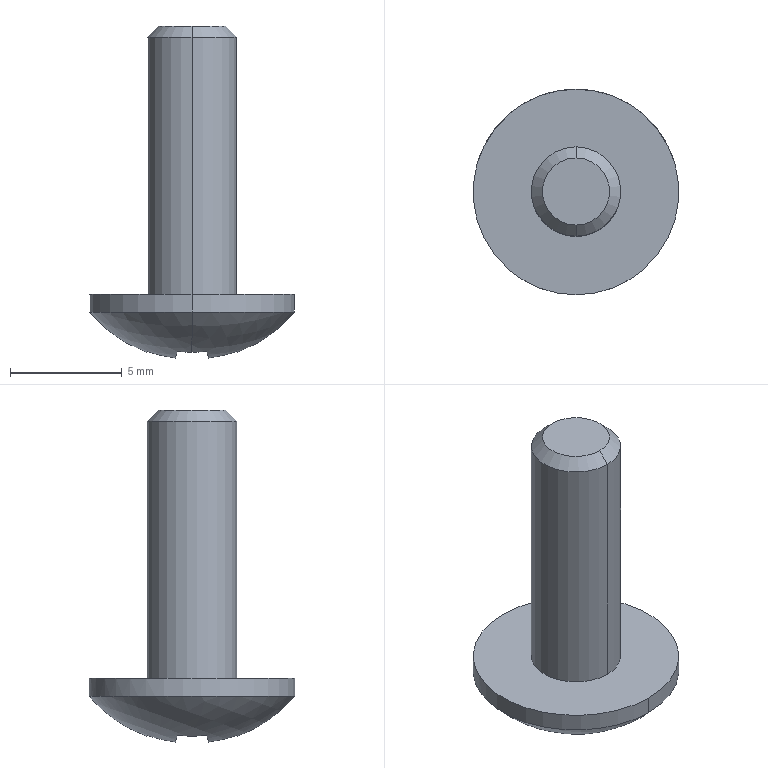Part | STEP file | MSBR-15_1_1_1_1 | 1 solid | 23 faces | box 9.2 x 9.2 x 14.856 mm | volume 268.703 mm3 | plane 15 | cylinder 4 | sphere 2 | cone 2 | commonest cylinder face diameters 4 x2 9.2 x2
STEP:
#1=CARTESIAN_POINT('',(0.,0.,0.));
#2=DIRECTION('',(0.,0.,1.));
#3=DIRECTION('',(1.,0.,0.));
#4=AXIS2_PLACEMENT_3D('',#1,#2,#3);
#5=CARTESIAN_POINT('',(0.,4.6,-18.7));
#6=VERTEX_POINT('',#5);
#7=CARTESIAN_POINT('',(0.,-4.6,-18.7));
#8=VERTEX_POINT('',#7);
#9=CARTESIAN_POINT('',(0.,0.,-18.7));
#10=DIRECTION('',(0.,0.,-1.));
#11=DIRECTION('',(0.,1.,0.));
#12=AXIS2_PLACEMENT_3D('',#9,#10,#11);
#13=CIRCLE('',#12,4.6);
#14=EDGE_CURVE('',#6,#8,#13,.T.);
#15=ORIENTED_EDGE('',*,*,#14,.F.);
#16=CARTESIAN_POINT('',(0.,4.6,-19.5));
#17=VERTEX_POINT('',#16);
#18=CARTESIAN_POINT('',(0.,4.6,-19.5));
#19=DIRECTION('',(0.,-0.000000001,1.));
#20=VECTOR('',#19,0.8);
#21=LINE('',#18,#20);
#22=EDGE_CURVE('',#17,#6,#21,.T.);
#23=ORIENTED_EDGE('',*,*,#22,.F.);
#24=CARTESIAN_POINT('',(0.,-4.6,-19.5));
#25=VERTEX_POINT('',#24);
#26=CARTESIAN_POINT('',(0.,0.,-19.5));
#27=DIRECTION('',(0.,0.,1.));
#28=DIRECTION('',(0.,-1.,0.));
#29=AXIS2_PLACEMENT_3D('',#26,#27,#28);
#30=CIRCLE('',#29,4.6);
#31=EDGE_CURVE('',#25,#17,#30,.T.);
#32=ORIENTED_EDGE('',*,*,#31,.F.);
#33=CARTESIAN_POINT('',(0.,-4.6,-18.7));
#34=DIRECTION('',(0.,-0.000000001,-1.));
#35=VECTOR('',#34,0.8);
#36=LINE('',#33,#35);
#37=EDGE_CURVE('',#8,#25,#36,.T.);
#38=ORIENTED_EDGE('',*,*,#37,.F.);
#39=EDGE_LOOP('',(#15,#23,#32,#38));
#40=FACE_OUTER_BOUND('',#39,.F.);
#41=CARTESIAN_POINT('',(0.,0.,-18.676));
#42=DIRECTION('',(0.,0.,-1.));
#43=DIRECTION('',(0.,1.,0.));
#44=AXIS2_PLACEMENT_3D('',#41,#42,#43);
#45=CYLINDRICAL_SURFACE('',#44,4.6);
#46=ADVANCED_FACE('',(#40),#45,.T.);
#47=CARTESIAN_POINT('',(0.,0.,-18.7));
#48=DIRECTION('',(0.,0.,-1.));
#49=DIRECTION('',(0.,-1.,0.));
#50=AXIS2_PLACEMENT_3D('',#47,#48,#49);
#51=CIRCLE('',#50,4.6);
#52=EDGE_CURVE('',#8,#6,#51,.T.);
#53=ORIENTED_EDGE('',*,*,#52,.T.);
#54=ORIENTED_EDGE('',*,*,#14,.T.);
#55=EDGE_LOOP('',(#53,#54));
#56=FACE_OUTER_BOUND('',#55,.F.);
#57=CARTESIAN_POINT('',(0.,-2.,-18.7));
#58=VERTEX_POINT('',#57);
#59=CARTESIAN_POINT('',(0.,2.,-18.7));
#60=VERTEX_POINT('',#59);
#61=CARTESIAN_POINT('',(0.,0.,-18.7));
#62=DIRECTION('',(0.,0.,1.));
#63=DIRECTION('',(0.,-1.,0.));
#64=AXIS2_PLACEMENT_3D('',#61,#62,#63);
#65=CIRCLE('',#64,2.);
#66=EDGE_CURVE('',#58,#60,#65,.T.);
#67=ORIENTED_EDGE('',*,*,#66,.T.);
#68=CARTESIAN_POINT('',(0.,0.,-18.7));
#69=DIRECTION('',(0.,0.,1.));
#70=DIRECTION('',(0.,1.,0.));
#71=AXIS2_PLACEMENT_3D('',#68,#69,#70);
#72=CIRCLE('',#71,2.);
#73=EDGE_CURVE('',#60,#58,#72,.T.);
#74=ORIENTED_EDGE('',*,*,#73,.T.);
#75=EDGE_LOOP('',(#67,#74));
#76=FACE_BOUND('',#75,.F.);
#77=CARTESIAN_POINT('',(0.,0.,-18.7));
#78=DIRECTION('',(0.,0.,1.));
#79=DIRECTION('',(0.,-1.,0.));
#80=AXIS2_PLACEMENT_3D('',#77,#78,#79);
#81=PLANE('',#80);
#82=ADVANCED_FACE('',(#56,#76),#81,.T.);
#83=ORIENTED_EDGE('',*,*,#37,.T.);
#84=CARTESIAN_POINT('',(0.,0.,-19.5));
#85=DIRECTION('',(0.,0.,1.));
#86=DIRECTION('',(0.,1.,0.));
#87=AXIS2_PLACEMENT_3D('',#84,#85,#86);
#88=CIRCLE('',#87,4.6);
#89=EDGE_CURVE('',#17,#25,#88,.T.);
#90=ORIENTED_EDGE('',*,*,#89,.F.);
#91=ORIENTED_EDGE('',*,*,#22,.T.);
#92=ORIENTED_EDGE('',*,*,#52,.F.);
#93=EDGE_LOOP('',(#83,#90,#91,#92));
#94=FACE_OUTER_BOUND('',#93,.F.);
#95=CARTESIAN_POINT('',(0.,0.,-18.676));
#96=DIRECTION('',(0.,0.,-1.));
#97=DIRECTION('',(0.,-1.,0.));
#98=AXIS2_PLACEMENT_3D('',#95,#96,#97);
#99=CYLINDRICAL_SURFACE('',#98,4.6);
#100=ADVANCED_FACE('',(#94),#99,.T.);
#101=ORIENTED_EDGE('',*,*,#89,.T.);
#102=CARTESIAN_POINT('',(0.,-2.03,-21.294));
#103=VERTEX_POINT('',#102);
#104=CARTESIAN_POINT('',(0.,0.,-15.648));
#105=DIRECTION('',(-1.,0.,0.));
#106=DIRECTION('',(0.,-0.3383,-0.941));
#107=AXIS2_PLACEMENT_3D('',#104,#105,#106);
#108=CIRCLE('',#107,6.);
#109=EDGE_CURVE('',#103,#25,#108,.T.);
#110=ORIENTED_EDGE('',*,*,#109,.F.);
#111=CARTESIAN_POINT('',(-0.669,-2.007,-21.262));
#112=VERTEX_POINT('',#111);
#113=CARTESIAN_POINT('',(0.,1.341,-16.613));
#114=DIRECTION('',(0.,-0.8115,0.5843));
#115=DIRECTION('',(-0.116,-0.5804,-0.8061));
#116=AXIS2_PLACEMENT_3D('',#113,#114,#115);
#117=CIRCLE('',#116,5.768);
#118=EDGE_CURVE('',#112,#103,#117,.T.);
#119=ORIENTED_EDGE('',*,*,#118,.F.);
#120=CARTESIAN_POINT('',(-0.7394,-0.7394,-21.556));
#121=VERTEX_POINT('',#120);
#122=CARTESIAN_POINT('',(0.6416,0.,-15.802));
#123=DIRECTION('',(-0.9724,0.,0.2334));
#124=DIRECTION('',(-0.2316,-0.124,-0.9649));
#125=AXIS2_PLACEMENT_3D('',#122,#123,#124);
#126=CIRCLE('',#125,5.964);
#127=EDGE_CURVE('',#121,#112,#126,.T.);
#128=ORIENTED_EDGE('',*,*,#127,.F.);
#129=CARTESIAN_POINT('',(-2.007,-0.669,-21.262));
#130=VERTEX_POINT('',#129);
#131=CARTESIAN_POINT('',(0.,0.6416,-15.802));
#132=DIRECTION('',(0.,-0.9724,0.2334));
#133=DIRECTION('',(-0.3365,-0.2198,-0.9157));
#134=AXIS2_PLACEMENT_3D('',#131,#132,#133);
#135=CIRCLE('',#134,5.964);
#136=EDGE_CURVE('',#130,#121,#135,.T.);
#137=ORIENTED_EDGE('',*,*,#136,.F.);
#138=CARTESIAN_POINT('',(-2.007,0.669,-21.262));
#139=VERTEX_POINT('',#138);
#140=CARTESIAN_POINT('',(1.341,0.,-16.613));
#141=DIRECTION('',(-0.8115,0.,0.5843));
#142=DIRECTION('',(-0.5804,0.116,-0.8061));
#143=AXIS2_PLACEMENT_3D('',#140,#141,#142);
#144=CIRCLE('',#143,5.768);
#145=EDGE_CURVE('',#139,#130,#144,.T.);
#146=ORIENTED_EDGE('',*,*,#145,.F.);
#147=CARTESIAN_POINT('',(-0.7394,0.7394,-21.556));
#148=VERTEX_POINT('',#147);
#149=CARTESIAN_POINT('',(0.,-0.6416,-15.802));
#150=DIRECTION('',(0.,-0.9724,-0.2334));
#151=DIRECTION('',(-0.3365,0.2198,-0.9157));
#152=AXIS2_PLACEMENT_3D('',#149,#150,#151);
#153=CIRCLE('',#152,5.964);
#154=EDGE_CURVE('',#139,#148,#153,.T.);
#155=ORIENTED_EDGE('',*,*,#154,.T.);
#156=CARTESIAN_POINT('',(-0.669,2.007,-21.262));
#157=VERTEX_POINT('',#156);
#158=CARTESIAN_POINT('',(0.6416,0.,-15.802));
#159=DIRECTION('',(0.9724,0.,-0.2334));
#160=DIRECTION('',(-0.2316,0.124,-0.9649));
#161=AXIS2_PLACEMENT_3D('',#158,#159,#160);
#162=CIRCLE('',#161,5.964);
#163=EDGE_CURVE('',#148,#157,#162,.T.);
#164=ORIENTED_EDGE('',*,*,#163,.T.);
#165=CARTESIAN_POINT('',(0.,2.03,-21.294));
#166=VERTEX_POINT('',#165);
#167=CARTESIAN_POINT('',(0.,-1.341,-16.613));
#168=DIRECTION('',(0.,0.8115,0.5843));
#169=DIRECTION('',(0.,0.5843,-0.8115));
#170=AXIS2_PLACEMENT_3D('',#167,#168,#169);
#171=CIRCLE('',#170,5.768);
#172=EDGE_CURVE('',#166,#157,#171,.T.);
#173=ORIENTED_EDGE('',*,*,#172,.F.);
#174=CARTESIAN_POINT('',(0.,0.,-15.648));
#175=DIRECTION('',(-1.,0.,0.));
#176=DIRECTION('',(0.,0.7667,-0.642));
#177=AXIS2_PLACEMENT_3D('',#174,#175,#176);
#178=CIRCLE('',#177,6.);
#179=EDGE_CURVE('',#17,#166,#178,.T.);
#180=ORIENTED_EDGE('',*,*,#179,.F.);
#181=EDGE_LOOP('',(#101,#110,#119,#128,#137,#146,#155,#164,#173,#180));
#182=FACE_OUTER_BOUND('',#181,.F.);
#183=CARTESIAN_POINT('',(0.,0.,-15.648));
#184=DIRECTION('',(0.,0.3383,-0.941));
#185=DIRECTION('',(0.,-0.941,-0.3383));
#186=AXIS2_PLACEMENT_3D('',#183,#184,#185);
#187=SPHERICAL_SURFACE('',#186,6.);
#188=ADVANCED_FACE('',(#182),#187,.T.);
#189=ORIENTED_EDGE('',*,*,#179,.T.);
#190=CARTESIAN_POINT('',(0.669,2.007,-21.262));
#191=VERTEX_POINT('',#190);
#192=CARTESIAN_POINT('',(0.,-1.341,-16.613));
#193=DIRECTION('',(0.,0.8115,0.5843));
#194=DIRECTION('',(0.116,0.5804,-0.8061));
#195=AXIS2_PLACEMENT_3D('',#192,#193,#194);
#196=CIRCLE('',#195,5.768);
#197=EDGE_CURVE('',#191,#166,#196,.T.);
#198=ORIENTED_EDGE('',*,*,#197,.F.);
#199=CARTESIAN_POINT('',(0.7394,0.7394,-21.556));
#200=VERTEX_POINT('',#199);
#201=CARTESIAN_POINT('',(-0.6416,0.,-15.802));
#202=DIRECTION('',(-0.9724,0.,-0.2334));
#203=DIRECTION('',(0.2198,0.3365,-0.9157));
#204=AXIS2_PLACEMENT_3D('',#201,#202,#203);
#205=CIRCLE('',#204,5.964);
#206=EDGE_CURVE('',#191,#200,#205,.T.);
#207=ORIENTED_EDGE('',*,*,#206,.T.);
#208=CARTESIAN_POINT('',(2.007,0.669,-21.262));
#209=VERTEX_POINT('',#208);
#210=CARTESIAN_POINT('',(0.,-0.6416,-15.802));
#211=DIRECTION('',(0.,-0.9724,-0.2334));
#212=DIRECTION('',(0.124,0.2316,-0.9649));
#213=AXIS2_PLACEMENT_3D('',#210,#211,#212);
#214=CIRCLE('',#213,5.964);
#215=EDGE_CURVE('',#200,#209,#214,.T.);
#216=ORIENTED_EDGE('',*,*,#215,.T.);
#217=CARTESIAN_POINT('',(2.007,-0.669,-21.262));
#218=VERTEX_POINT('',#217);
#219=CARTESIAN_POINT('',(-1.341,0.,-16.613));
#220=DIRECTION('',(-0.8115,0.,-0.5843));
#221=DIRECTION('',(0.5804,0.116,-0.8061));
#222=AXIS2_PLACEMENT_3D('',#219,#220,#221);
#223=CIRCLE('',#222,5.768);
#224=EDGE_CURVE('',#209,#218,#223,.T.);
#225=ORIENTED_EDGE('',*,*,#224,.T.);
#226=CARTESIAN_POINT('',(0.7394,-0.7394,-21.556));
#227=VERTEX_POINT('',#226);
#228=CARTESIAN_POINT('',(0.,0.6416,-15.802));
#229=DIRECTION('',(0.,-0.9724,0.2334));
#230=DIRECTION('',(0.124,-0.2316,-0.9649));
#231=AXIS2_PLACEMENT_3D('',#228,#229,#230);
#232=CIRCLE('',#231,5.964);
#233=EDGE_CURVE('',#227,#218,#232,.T.);
#234=ORIENTED_EDGE('',*,*,#233,.F.);
#235=CARTESIAN_POINT('',(0.669,-2.007,-21.262));
#236=VERTEX_POINT('',#235);
#237=CARTESIAN_POINT('',(-0.6416,0.,-15.802));
#238=DIRECTION('',(0.9724,0.,0.2334));
#239=DIRECTION('',(0.2198,-0.3365,-0.9157));
#240=AXIS2_PLACEMENT_3D('',#237,#238,#239);
#241=CIRCLE('',#240,5.964);
#242=EDGE_CURVE('',#236,#227,#241,.T.);
#243=ORIENTED_EDGE('',*,*,#242,.F.);
#244=CARTESIAN_POINT('',(0.,1.341,-16.613));
#245=DIRECTION('',(0.,-0.8115,0.5843));
#246=DIRECTION('',(0.,-0.5843,-0.8115));
#247=AXIS2_PLACEMENT_3D('',#244,#245,#246);
#248=CIRCLE('',#247,5.768);
#249=EDGE_CURVE('',#103,#236,#248,.T.);
#250=ORIENTED_EDGE('',*,*,#249,.F.);
#251=ORIENTED_EDGE('',*,*,#109,.T.);
#252=ORIENTED_EDGE('',*,*,#31,.T.);
#253=EDGE_LOOP('',(#189,#198,#207,#216,#225,#234,#243,#250,#251,#252));
#254=FACE_OUTER_BOUND('',#253,.F.);
#255=CARTESIAN_POINT('',(0.,0.,-15.648));
#256=DIRECTION('',(0.,0.3383,-0.941));
#257=DIRECTION('',(0.,0.941,0.3383));
#258=AXIS2_PLACEMENT_3D('',#255,#256,#257);
#259=SPHERICAL_SURFACE('',#258,6.);
#260=ADVANCED_FACE('',(#254),#259,.T.);
#261=CARTESIAN_POINT('',(0.15,0.45,-19.1));
#262=VERTEX_POINT('',#261);
#263=CARTESIAN_POINT('',(0.669,2.007,-21.262));
#264=DIRECTION('',(-0.1912,-0.5735,0.7966));
#265=VECTOR('',#264,2.715);
#266=LINE('',#263,#265);
#267=EDGE_CURVE('',#191,#262,#266,.T.);
#268=ORIENTED_EDGE('',*,*,#267,.F.);
#269=ORIENTED_EDGE('',*,*,#197,.T.);
#270=ORIENTED_EDGE('',*,*,#172,.T.);
#271=CARTESIAN_POINT('',(-0.15,0.45,-19.1));
#272=VERTEX_POINT('',#271);
#273=CARTESIAN_POINT('',(-0.15,0.45,-19.1));
#274=DIRECTION('',(-0.1912,0.5735,-0.7966));
#275=VECTOR('',#274,2.715);
#276=LINE('',#273,#275);
#277=EDGE_CURVE('',#272,#157,#276,.T.);
#278=ORIENTED_EDGE('',*,*,#277,.F.);
#279=CARTESIAN_POINT('',(0.15,0.45,-19.1));
#280=DIRECTION('',(-1.,0.,0.));
#281=VECTOR('',#280,0.3);
#282=LINE('',#279,#281);
#283=EDGE_CURVE('',#262,#272,#282,.T.);
#284=ORIENTED_EDGE('',*,*,#283,.F.);
#285=EDGE_LOOP('',(#268,#269,#270,#278,#284));
#286=FACE_OUTER_BOUND('',#285,.F.);
#287=CARTESIAN_POINT('',(0.,1.24,-20.197));
#288=DIRECTION('',(0.,0.8115,0.5843));
#289=DIRECTION('',(1.,0.,0.));
#290=AXIS2_PLACEMENT_3D('',#287,#288,#289);
#291=PLANE('',#290);
#292=ADVANCED_FACE('',(#286),#291,.F.);
#293=CARTESIAN_POINT('',(0.15,0.15,-19.1));
#294=VERTEX_POINT('',#293);
#295=CARTESIAN_POINT('',(0.15,0.15,-19.1));
#296=DIRECTION('',(0.,1.,0.));
#297=VECTOR('',#296,0.3);
#298=LINE('',#295,#297);
#299=EDGE_CURVE('',#294,#262,#298,.T.);
#300=ORIENTED_EDGE('',*,*,#299,.F.);
#301=CARTESIAN_POINT('',(0.7394,0.7394,-21.556));
#302=DIRECTION('',(-0.2273,-0.2273,0.9469));
#303=VECTOR('',#302,2.594);
#304=LINE('',#301,#303);
#305=EDGE_CURVE('',#200,#294,#304,.T.);
#306=ORIENTED_EDGE('',*,*,#305,.F.);
#307=ORIENTED_EDGE('',*,*,#206,.F.);
#308=ORIENTED_EDGE('',*,*,#267,.T.);
#309=EDGE_LOOP('',(#300,#306,#307,#308));
#310=FACE_OUTER_BOUND('',#309,.F.);
#311=CARTESIAN_POINT('',(0.4447,1.078,-20.328));
#312=DIRECTION('',(0.9724,0.,0.2334));
#313=DIRECTION('',(0.,-1.,0.));
#314=AXIS2_PLACEMENT_3D('',#311,#312,#313);
#315=PLANE('',#314);
#316=ADVANCED_FACE('',(#310),#315,.F.);
#317=CARTESIAN_POINT('',(-0.45,0.15,-19.1));
#318=VERTEX_POINT('',#317);
#319=CARTESIAN_POINT('',(-0.15,0.15,-19.1));
#320=VERTEX_POINT('',#319);
#321=CARTESIAN_POINT('',(-0.45,0.15,-19.1));
#322=DIRECTION('',(1.,0.,0.));
#323=VECTOR('',#322,0.3);
#324=LINE('',#321,#323);
#325=EDGE_CURVE('',#318,#320,#324,.T.);
#326=ORIENTED_EDGE('',*,*,#325,.F.);
#327=CARTESIAN_POINT('',(-0.45,-0.15,-19.1));
#328=VERTEX_POINT('',#327);
#329=CARTESIAN_POINT('',(-0.45,-0.15,-19.1));
#330=DIRECTION('',(0.,1.,0.));
#331=VECTOR('',#330,0.3);
#332=LINE('',#329,#331);
#333=EDGE_CURVE('',#328,#318,#332,.T.);
#334=ORIENTED_EDGE('',*,*,#333,.F.);
#335=CARTESIAN_POINT('',(-0.15,-0.15,-19.1));
#336=VERTEX_POINT('',#335);
#337=CARTESIAN_POINT('',(-0.15,-0.15,-19.1));
#338=DIRECTION('',(-1.,0.,0.));
#339=VECTOR('',#338,0.3);
#340=LINE('',#337,#339);
#341=EDGE_CURVE('',#336,#328,#340,.T.);
#342=ORIENTED_EDGE('',*,*,#341,.F.);
#343=CARTESIAN_POINT('',(-0.15,-0.45,-19.1));
#344=VERTEX_POINT('',#343);
#345=CARTESIAN_POINT('',(-0.15,-0.45,-19.1));
#346=DIRECTION('',(0.,1.,0.));
#347=VECTOR('',#346,0.3);
#348=LINE('',#345,#347);
#349=EDGE_CURVE('',#344,#336,#348,.T.);
#350=ORIENTED_EDGE('',*,*,#349,.F.);
#351=CARTESIAN_POINT('',(0.15,-0.45,-19.1));
#352=VERTEX_POINT('',#351);
#353=CARTESIAN_POINT('',(0.15,-0.45,-19.1));
#354=DIRECTION('',(-1.,0.,0.));
#355=VECTOR('',#354,0.3);
#356=LINE('',#353,#355);
#357=EDGE_CURVE('',#352,#344,#356,.T.);
#358=ORIENTED_EDGE('',*,*,#357,.F.);
#359=CARTESIAN_POINT('',(0.15,-0.15,-19.1));
#360=VERTEX_POINT('',#359);
#361=CARTESIAN_POINT('',(0.15,-0.15,-19.1));
#362=DIRECTION('',(0.,-1.,0.));
#363=VECTOR('',#362,0.3);
#364=LINE('',#361,#363);
#365=EDGE_CURVE('',#360,#352,#364,.T.);
#366=ORIENTED_EDGE('',*,*,#365,.F.);
#367=CARTESIAN_POINT('',(0.45,-0.15,-19.1));
#368=VERTEX_POINT('',#367);
#369=CARTESIAN_POINT('',(0.45,-0.15,-19.1));
#370=DIRECTION('',(-1.,0.,0.));
#371=VECTOR('',#370,0.3);
#372=LINE('',#369,#371);
#373=EDGE_CURVE('',#368,#360,#372,.T.);
#374=ORIENTED_EDGE('',*,*,#373,.F.);
#375=CARTESIAN_POINT('',(0.45,0.15,-19.1));
#376=VERTEX_POINT('',#375);
#377=CARTESIAN_POINT('',(0.45,0.15,-19.1));
#378=DIRECTION('',(0.,-1.,0.));
#379=VECTOR('',#378,0.3);
#380=LINE('',#377,#379);
#381=EDGE_CURVE('',#376,#368,#380,.T.);
#382=ORIENTED_EDGE('',*,*,#381,.F.);
#383=CARTESIAN_POINT('',(0.15,0.15,-19.1));
#384=DIRECTION('',(1.,0.,0.));
#385=VECTOR('',#384,0.3);
#386=LINE('',#383,#385);
#387=EDGE_CURVE('',#294,#376,#386,.T.);
#388=ORIENTED_EDGE('',*,*,#387,.F.);
#389=ORIENTED_EDGE('',*,*,#299,.T.);
#390=ORIENTED_EDGE('',*,*,#283,.T.);
#391=CARTESIAN_POINT('',(-0.15,0.15,-19.1));
#392=DIRECTION('',(0.,1.,0.));
#393=VECTOR('',#392,0.3);
#394=LINE('',#391,#393);
#395=EDGE_CURVE('',#320,#272,#394,.T.);
#396=ORIENTED_EDGE('',*,*,#395,.F.);
#397=EDGE_LOOP('',(#326,#334,#342,#350,#358,#366,#374,#382,#388,#389,#390,#396));
#398=FACE_OUTER_BOUND('',#397,.F.);
#399=CARTESIAN_POINT('',(0.,0.,-19.1));
#400=DIRECTION('',(0.,0.,1.));
#401=DIRECTION('',(0.,-1.,0.));
#402=AXIS2_PLACEMENT_3D('',#399,#400,#401);
#403=PLANE('',#402);
#404=ADVANCED_FACE('',(#398),#403,.F.);
#405=ORIENTED_EDGE('',*,*,#325,.T.);
#406=CARTESIAN_POINT('',(-0.7394,0.7394,-21.556));
#407=DIRECTION('',(0.2273,-0.2273,0.9469));
#408=VECTOR('',#407,2.594);
#409=LINE('',#406,#408);
#410=EDGE_CURVE('',#148,#320,#409,.T.);
#411=ORIENTED_EDGE('',*,*,#410,.F.);
#412=ORIENTED_EDGE('',*,*,#154,.F.);
#413=CARTESIAN_POINT('',(-0.45,0.15,-19.1));
#414=DIRECTION('',(-0.5735,0.1912,-0.7966));
#415=VECTOR('',#414,2.715);
#416=LINE('',#413,#415);
#417=EDGE_CURVE('',#318,#139,#416,.T.);
#418=ORIENTED_EDGE('',*,*,#417,.F.);
#419=EDGE_LOOP('',(#405,#411,#412,#418));
#420=FACE_OUTER_BOUND('',#419,.F.);
#421=CARTESIAN_POINT('',(-1.078,0.4447,-20.328));
#422=DIRECTION('',(0.,0.9724,0.2334));
#423=DIRECTION('',(1.,0.,0.));
#424=AXIS2_PLACEMENT_3D('',#421,#422,#423);
#425=PLANE('',#424);
#426=ADVANCED_FACE('',(#420),#425,.F.);
#427=ORIENTED_EDGE('',*,*,#395,.T.);
#428=ORIENTED_EDGE('',*,*,#277,.T.);
#429=ORIENTED_EDGE('',*,*,#163,.F.);
#430=ORIENTED_EDGE('',*,*,#410,.T.);
#431=EDGE_LOOP('',(#427,#428,#429,#430));
#432=FACE_OUTER_BOUND('',#431,.F.);
#433=CARTESIAN_POINT('',(-0.4447,1.078,-20.328));
#434=DIRECTION('',(0.9724,0.,-0.2334));
#435=DIRECTION('',(0.,1.,0.));
#436=AXIS2_PLACEMENT_3D('',#433,#434,#435);
#437=PLANE('',#436);
#438=ADVANCED_FACE('',(#432),#437,.T.);
#439=ORIENTED_EDGE('',*,*,#333,.T.);
#440=ORIENTED_EDGE('',*,*,#417,.T.);
#441=ORIENTED_EDGE('',*,*,#145,.T.);
#442=CARTESIAN_POINT('',(-0.45,-0.15,-19.1));
#443=DIRECTION('',(-0.5735,-0.1912,-0.7966));
#444=VECTOR('',#443,2.715);
#445=LINE('',#442,#444);
#446=EDGE_CURVE('',#328,#130,#445,.T.);
#447=ORIENTED_EDGE('',*,*,#446,.F.);
#448=EDGE_LOOP('',(#439,#440,#441,#447));
#449=FACE_OUTER_BOUND('',#448,.F.);
#450=CARTESIAN_POINT('',(-1.24,0.,-20.197));
#451=DIRECTION('',(0.8115,0.,-0.5843));
#452=DIRECTION('',(0.,1.,0.));
#453=AXIS2_PLACEMENT_3D('',#450,#451,#452);
#454=PLANE('',#453);
#455=ADVANCED_FACE('',(#449),#454,.T.);
#456=ORIENTED_EDGE('',*,*,#341,.T.);
#457=ORIENTED_EDGE('',*,*,#446,.T.);
#458=ORIENTED_EDGE('',*,*,#136,.T.);
#459=CARTESIAN_POINT('',(-0.15,-0.15,-19.1));
#460=DIRECTION('',(-0.2273,-0.2273,-0.9469));
#461=VECTOR('',#460,2.594);
#462=LINE('',#459,#461);
#463=EDGE_CURVE('',#336,#121,#462,.T.);
#464=ORIENTED_EDGE('',*,*,#463,.F.);
#465=EDGE_LOOP('',(#456,#457,#458,#464));
#466=FACE_OUTER_BOUND('',#465,.F.);
#467=CARTESIAN_POINT('',(-1.078,-0.4447,-20.328));
#468=DIRECTION('',(0.,0.9724,-0.2334));
#469=DIRECTION('',(-1.,0.,0.));
#470=AXIS2_PLACEMENT_3D('',#467,#468,#469);
#471=PLANE('',#470);
#472=ADVANCED_FACE('',(#466),#471,.T.);
#473=ORIENTED_EDGE('',*,*,#349,.T.);
#474=ORIENTED_EDGE('',*,*,#463,.T.);
#475=ORIENTED_EDGE('',*,*,#127,.T.);
#476=CARTESIAN_POINT('',(-0.15,-0.45,-19.1));
#477=DIRECTION('',(-0.1912,-0.5735,-0.7966));
#478=VECTOR('',#477,2.715);
#479=LINE('',#476,#478);
#480=EDGE_CURVE('',#344,#112,#479,.T.);
#481=ORIENTED_EDGE('',*,*,#480,.F.);
#482=EDGE_LOOP('',(#473,#474,#475,#481));
#483=FACE_OUTER_BOUND('',#482,.F.);
#484=CARTESIAN_POINT('',(-0.4447,-1.078,-20.328));
#485=DIRECTION('',(0.9724,0.,-0.2334));
#486=DIRECTION('',(0.,1.,0.));
#487=AXIS2_PLACEMENT_3D('',#484,#485,#486);
#488=PLANE('',#487);
#489=ADVANCED_FACE('',(#483),#488,.T.);
#490=ORIENTED_EDGE('',*,*,#357,.T.);
#491=ORIENTED_EDGE('',*,*,#480,.T.);
#492=ORIENTED_EDGE('',*,*,#118,.T.);
#493=ORIENTED_EDGE('',*,*,#249,.T.);
#494=CARTESIAN_POINT('',(0.15,-0.45,-19.1));
#495=DIRECTION('',(0.1912,-0.5735,-0.7966));
#496=VECTOR('',#495,2.715);
#497=LINE('',#494,#496);
#498=EDGE_CURVE('',#352,#236,#497,.T.);
#499=ORIENTED_EDGE('',*,*,#498,.F.);
#500=EDGE_LOOP('',(#490,#491,#492,#493,#499));
#501=FACE_OUTER_BOUND('',#500,.F.);
#502=CARTESIAN_POINT('',(0.,-1.24,-20.197));
#503=DIRECTION('',(0.,0.8115,-0.5843));
#504=DIRECTION('',(-1.,0.,0.));
#505=AXIS2_PLACEMENT_3D('',#502,#503,#504);
#506=PLANE('',#505);
#507=ADVANCED_FACE('',(#501),#506,.T.);
#508=ORIENTED_EDGE('',*,*,#365,.T.);
#509=ORIENTED_EDGE('',*,*,#498,.T.);
#510=ORIENTED_EDGE('',*,*,#242,.T.);
#511=CARTESIAN_POINT('',(0.15,-0.15,-19.1));
#512=DIRECTION('',(0.2273,-0.2273,-0.9469));
#513=VECTOR('',#512,2.594);
#514=LINE('',#511,#513);
#515=EDGE_CURVE('',#360,#227,#514,.T.);
#516=ORIENTED_EDGE('',*,*,#515,.F.);
#517=EDGE_LOOP('',(#508,#509,#510,#516));
#518=FACE_OUTER_BOUND('',#517,.F.);
#519=CARTESIAN_POINT('',(0.4447,-1.078,-20.328));
#520=DIRECTION('',(0.9724,0.,0.2334));
#521=DIRECTION('',(0.,-1.,0.));
#522=AXIS2_PLACEMENT_3D('',#519,#520,#521);
#523=PLANE('',#522);
#524=ADVANCED_FACE('',(#518),#523,.F.);
#525=ORIENTED_EDGE('',*,*,#373,.T.);
#526=ORIENTED_EDGE('',*,*,#515,.T.);
#527=ORIENTED_EDGE('',*,*,#233,.T.);
#528=CARTESIAN_POINT('',(0.45,-0.15,-19.1));
#529=DIRECTION('',(0.5735,-0.1912,-0.7966));
#530=VECTOR('',#529,2.715);
#531=LINE('',#528,#530);
#532=EDGE_CURVE('',#368,#218,#531,.T.);
#533=ORIENTED_EDGE('',*,*,#532,.F.);
#534=EDGE_LOOP('',(#525,#526,#527,#533));
#535=FACE_OUTER_BOUND('',#534,.F.);
#536=CARTESIAN_POINT('',(1.078,-0.4447,-20.328));
#537=DIRECTION('',(0.,0.9724,-0.2334));
#538=DIRECTION('',(-1.,0.,0.));
#539=AXIS2_PLACEMENT_3D('',#536,#537,#538);
#540=PLANE('',#539);
#541=ADVANCED_FACE('',(#535),#540,.T.);
#542=ORIENTED_EDGE('',*,*,#381,.T.);
#543=ORIENTED_EDGE('',*,*,#532,.T.);
#544=ORIENTED_EDGE('',*,*,#224,.F.);
#545=CARTESIAN_POINT('',(0.45,0.15,-19.1));
#546=DIRECTION('',(0.5735,0.1912,-0.7966));
#547=VECTOR('',#546,2.715);
#548=LINE('',#545,#547);
#549=EDGE_CURVE('',#376,#209,#548,.T.);
#550=ORIENTED_EDGE('',*,*,#549,.F.);
#551=EDGE_LOOP('',(#542,#543,#544,#550));
#552=FACE_OUTER_BOUND('',#551,.F.);
#553=CARTESIAN_POINT('',(1.24,0.,-20.197));
#554=DIRECTION('',(0.8115,0.,0.5843));
#555=DIRECTION('',(0.,-1.,0.));
#556=AXIS2_PLACEMENT_3D('',#553,#554,#555);
#557=PLANE('',#556);
#558=ADVANCED_FACE('',(#552),#557,.F.);
#559=ORIENTED_EDGE('',*,*,#387,.T.);
#560=ORIENTED_EDGE('',*,*,#549,.T.);
#561=ORIENTED_EDGE('',*,*,#215,.F.);
#562=ORIENTED_EDGE('',*,*,#305,.T.);
#563=EDGE_LOOP('',(#559,#560,#561,#562));
#564=FACE_OUTER_BOUND('',#563,.F.);
#565=CARTESIAN_POINT('',(1.078,0.4447,-20.328));
#566=DIRECTION('',(0.,0.9724,0.2334));
#567=DIRECTION('',(1.,0.,0.));
#568=AXIS2_PLACEMENT_3D('',#565,#566,#567);
#569=PLANE('',#568);
#570=ADVANCED_FACE('',(#564),#569,.F.);
#571=CARTESIAN_POINT('',(0.,2.,-7.2));
#572=VERTEX_POINT('',#571);
#573=CARTESIAN_POINT('',(0.,-2.,-7.2));
#574=VERTEX_POINT('',#573);
#575=CARTESIAN_POINT('',(0.,0.,-7.2));
#576=DIRECTION('',(0.000000001,0.,-1.));
#577=DIRECTION('',(0.,1.,0.));
#578=AXIS2_PLACEMENT_3D('',#575,#576,#577);
#579=CIRCLE('',#578,2.);
#580=EDGE_CURVE('',#572,#574,#579,.T.);
#581=ORIENTED_EDGE('',*,*,#580,.F.);
#582=CARTESIAN_POINT('',(0.,2.,-18.7));
#583=DIRECTION('',(0.,0.,1.));
#584=VECTOR('',#583,11.5);
#585=LINE('',#582,#584);
#586=EDGE_CURVE('',#60,#572,#585,.T.);
#587=ORIENTED_EDGE('',*,*,#586,.F.);
#588=ORIENTED_EDGE('',*,*,#66,.F.);
#589=CARTESIAN_POINT('',(0.,-2.,-7.2));
#590=DIRECTION('',(0.,0.,-1.));
#591=VECTOR('',#590,11.5);
#592=LINE('',#589,#591);
#593=EDGE_CURVE('',#574,#58,#592,.T.);
#594=ORIENTED_EDGE('',*,*,#593,.F.);
#595=EDGE_LOOP('',(#581,#587,#588,#594));
#596=FACE_OUTER_BOUND('',#595,.F.);
#597=CARTESIAN_POINT('',(0.,0.,-6.97));
#598=DIRECTION('',(0.,0.,-1.));
#599=DIRECTION('',(0.,1.,0.));
#600=AXIS2_PLACEMENT_3D('',#597,#598,#599);
#601=CYLINDRICAL_SURFACE('',#600,2.);
#602=ADVANCED_FACE('',(#596),#601,.T.);
#603=CARTESIAN_POINT('',(0.,1.5,-6.7));
#604=VERTEX_POINT('',#603);
#605=CARTESIAN_POINT('',(0.,-1.5,-6.7));
#606=VERTEX_POINT('',#605);
#607=CARTESIAN_POINT('',(0.,0.,-6.7));
#608=DIRECTION('',(0.000000001,0.,-1.));
#609=DIRECTION('',(0.,1.,0.));
#610=AXIS2_PLACEMENT_3D('',#607,#608,#609);
#611=CIRCLE('',#610,1.5);
#612=EDGE_CURVE('',#604,#606,#611,.T.);
#613=ORIENTED_EDGE('',*,*,#612,.F.);
#614=CARTESIAN_POINT('',(0.,2.,-7.2));
#615=DIRECTION('',(0.,-0.7071,0.7071));
#616=VECTOR('',#615,0.7071);
#617=LINE('',#614,#616);
#618=EDGE_CURVE('',#572,#604,#617,.T.);
#619=ORIENTED_EDGE('',*,*,#618,.F.);
#620=ORIENTED_EDGE('',*,*,#580,.T.);
#621=CARTESIAN_POINT('',(0.,-1.5,-6.7));
#622=DIRECTION('',(0.,-0.7071,-0.7071));
#623=VECTOR('',#622,0.7071);
#624=LINE('',#621,#623);
#625=EDGE_CURVE('',#606,#574,#624,.T.);
#626=ORIENTED_EDGE('',*,*,#625,.F.);
#627=EDGE_LOOP('',(#613,#619,#620,#626));
#628=FACE_OUTER_BOUND('',#627,.F.);
#629=CARTESIAN_POINT('',(0.,0.,-6.95));
#630=DIRECTION('',(0.000000001,0.,-1.));
#631=DIRECTION('',(0.,-1.,0.));
#632=AXIS2_PLACEMENT_3D('',#629,#630,#631);
#633=CONICAL_SURFACE('',#632,1.75,45.);
#634=ADVANCED_FACE('',(#628),#633,.T.);
#635=CARTESIAN_POINT('',(0.,0.,-6.7));
#636=DIRECTION('',(-0.000000001,0.,-1.));
#637=DIRECTION('',(0.,-1.,0.));
#638=AXIS2_PLACEMENT_3D('',#635,#636,#637);
#639=CIRCLE('',#638,1.5);
#640=EDGE_CURVE('',#606,#604,#639,.T.);
#641=ORIENTED_EDGE('',*,*,#640,.T.);
#642=ORIENTED_EDGE('',*,*,#612,.T.);
#643=EDGE_LOOP('',(#641,#642));
#644=FACE_OUTER_BOUND('',#643,.F.);
#645=CARTESIAN_POINT('',(0.,0.,-6.7));
#646=DIRECTION('',(0.,0.,1.));
#647=DIRECTION('',(0.,-1.,0.));
#648=AXIS2_PLACEMENT_3D('',#645,#646,#647);
#649=PLANE('',#648);
#650=ADVANCED_FACE('',(#644),#649,.T.);
#651=ORIENTED_EDGE('',*,*,#625,.T.);
#652=CARTESIAN_POINT('',(0.,0.,-7.2));
#653=DIRECTION('',(-0.000000001,0.,-1.));
#654=DIRECTION('',(0.,-1.,0.));
#655=AXIS2_PLACEMENT_3D('',#652,#653,#654);
#656=CIRCLE('',#655,2.);
#657=EDGE_CURVE('',#574,#572,#656,.T.);
#658=ORIENTED_EDGE('',*,*,#657,.T.);
#659=ORIENTED_EDGE('',*,*,#618,.T.);
#660=ORIENTED_EDGE('',*,*,#640,.F.);
#661=EDGE_LOOP('',(#651,#658,#659,#660));
#662=FACE_OUTER_BOUND('',#661,.F.);
#663=CARTESIAN_POINT('',(0.,0.,-6.95));
#664=DIRECTION('',(-0.000000001,0.,-1.));
#665=DIRECTION('',(0.,1.,0.));
#666=AXIS2_PLACEMENT_3D('',#663,#664,#665);
#667=CONICAL_SURFACE('',#666,1.75,45.);
#668=ADVANCED_FACE('',(#662),#667,.T.);
#669=ORIENTED_EDGE('',*,*,#593,.T.);
#670=ORIENTED_EDGE('',*,*,#73,.F.);
#671=ORIENTED_EDGE('',*,*,#586,.T.);
#672=ORIENTED_EDGE('',*,*,#657,.F.);
#673=EDGE_LOOP('',(#669,#670,#671,#672));
#674=FACE_OUTER_BOUND('',#673,.F.);
#675=CARTESIAN_POINT('',(0.,0.,-6.97));
#676=DIRECTION('',(0.,0.,-1.));
#677=DIRECTION('',(0.,-1.,0.));
#678=AXIS2_PLACEMENT_3D('',#675,#676,#677);
#679=CYLINDRICAL_SURFACE('',#678,2.);
#680=ADVANCED_FACE('',(#674),#679,.T.);
#681=CLOSED_SHELL('',(#46,#82,#100,#188,#260,#292,#316,#404,#426,#438,#455,#472,#489,#507,#524,#541,#558,#570,#602,#634,#650,#668,#680));
#682=MANIFOLD_SOLID_BREP('',#681);
#683=(LENGTH_UNIT()NAMED_UNIT(*)SI_UNIT(.MILLI.,.METRE.));
#684=UNCERTAINTY_MEASURE_WITH_UNIT(LENGTH_MEASURE(0.002151),#683,'','');
#685=(NAMED_UNIT(*)PLANE_ANGLE_UNIT()SI_UNIT($,.RADIAN.));
#686=PLANE_ANGLE_MEASURE_WITH_UNIT(PLANE_ANGLE_MEASURE(0.01745),#685);
#687=(CONVERSION_BASED_UNIT('DEGREE',#686)NAMED_UNIT(*)PLANE_ANGLE_UNIT());
#688=(NAMED_UNIT(*)SI_UNIT($,.STERADIAN.)SOLID_ANGLE_UNIT());
#689=(GEOMETRIC_REPRESENTATION_CONTEXT(3)GLOBAL_UNCERTAINTY_ASSIGNED_CONTEXT((#684))GLOBAL_UNIT_ASSIGNED_CONTEXT((#683,#687,#688))REPRESENTATION_CONTEXT('',''));
#690=ADVANCED_BREP_SHAPE_REPRESENTATION('',(#4,#682),#689);